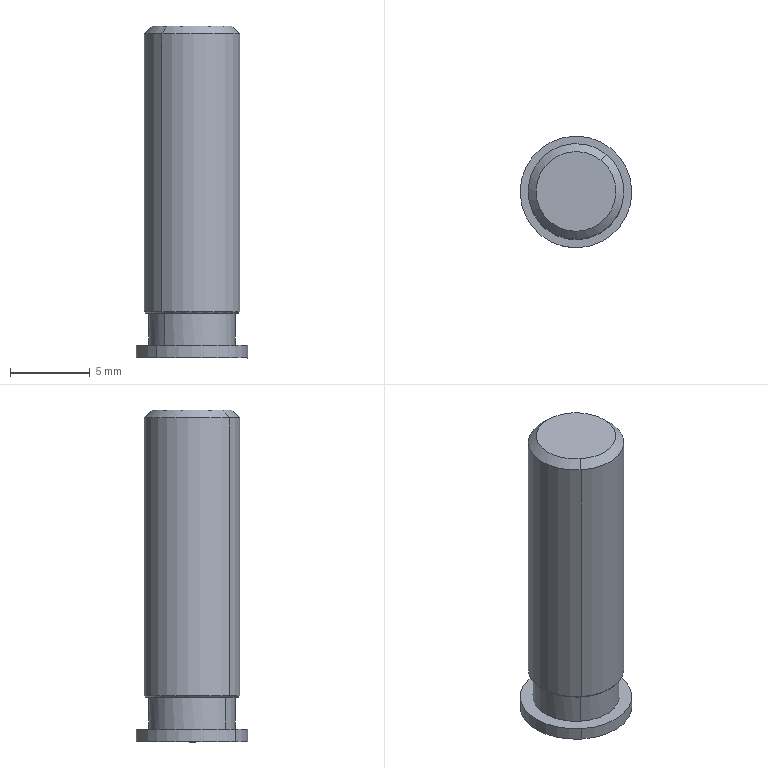Part | 1 solid | 14 faces | box 7 x 7 x 20.8 mm | volume 583.212 mm3 | other 7 | cylinder 6 | plane 1 | commonest cylinder face diameters 5.4 x2 6 x2 7 x2